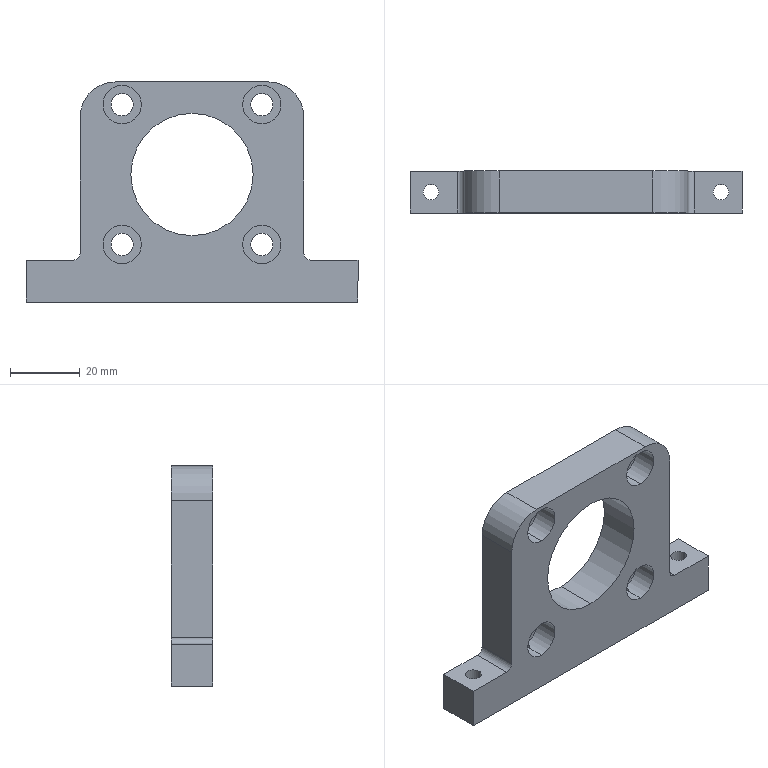Part | SolidWorks | features HoleWzd 7, ICE 3, Fillet 2, Extrusion 1 | 1 solid | 48 faces | box 95 x 12 x 63 mm | volume 36710 mm3 | cylinder 30 | plane 14 | cone 4 | commonest cylinder face diameters 6.4 x8 11 x8 4.5 x4 5 x4 4 x2 20 x2